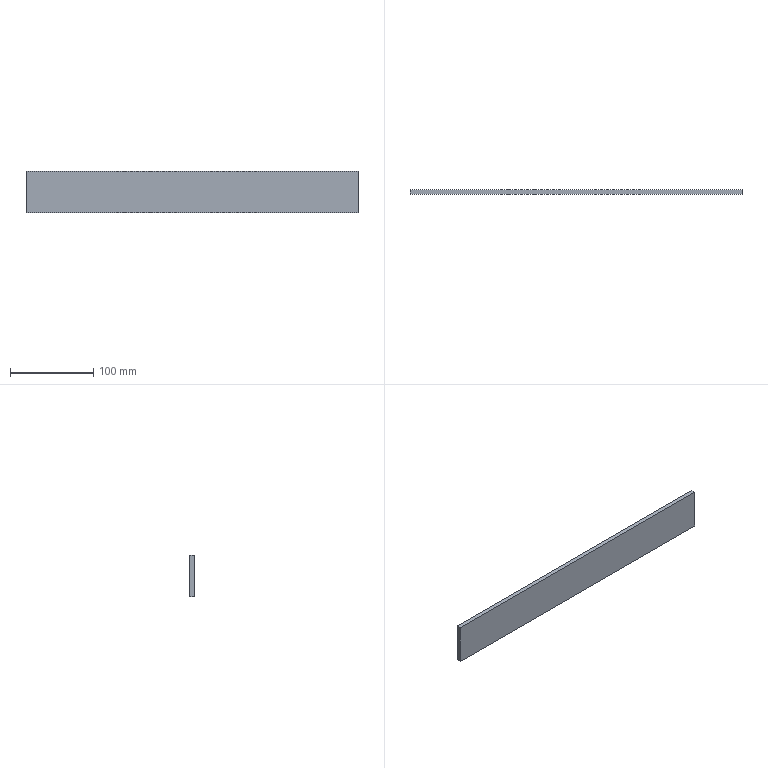Part | SolidWorks | features Extrusion 1 | 1 solid | 6 faces | box 400 x 5 x 50 mm | volume 100000 mm3 | plane 6
STEP:
#1=CARTESIAN_POINT('',(-200.,0.,-25.));
#2=VERTEX_POINT('',#1);
#3=CARTESIAN_POINT('',(-200.,0.,25.));
#4=VERTEX_POINT('',#3);
#5=CARTESIAN_POINT('',(-200.,0.,-25.));
#6=DIRECTION('',(0.,0.,1.));
#7=VECTOR('',#6,1000.);
#8=LINE('',#5,#7);
#9=EDGE_CURVE('',#2,#4,#8,.T.);
#10=ORIENTED_EDGE('',*,*,#9,.T.);
#11=CARTESIAN_POINT('',(-200.,5.,25.));
#12=VERTEX_POINT('',#11);
#13=CARTESIAN_POINT('',(-200.,5.,25.));
#14=DIRECTION('',(0.,-1.,0.));
#15=VECTOR('',#14,1000.);
#16=LINE('',#13,#15);
#17=EDGE_CURVE('',#12,#4,#16,.T.);
#18=ORIENTED_EDGE('',*,*,#17,.F.);
#19=CARTESIAN_POINT('',(-200.,5.,-25.));
#20=VERTEX_POINT('',#19);
#21=CARTESIAN_POINT('',(-200.,5.,-25.));
#22=DIRECTION('',(0.,0.,1.));
#23=VECTOR('',#22,1000.);
#24=LINE('',#21,#23);
#25=EDGE_CURVE('',#20,#12,#24,.T.);
#26=ORIENTED_EDGE('',*,*,#25,.F.);
#27=CARTESIAN_POINT('',(-200.,5.,-25.));
#28=DIRECTION('',(0.,-1.,0.));
#29=VECTOR('',#28,1000.);
#30=LINE('',#27,#29);
#31=EDGE_CURVE('',#20,#2,#30,.T.);
#32=ORIENTED_EDGE('',*,*,#31,.T.);
#33=EDGE_LOOP('',(#10,#18,#26,#32));
#34=FACE_OUTER_BOUND('',#33,.T.);
#35=CARTESIAN_POINT('',(-200.,5.,-25.));
#36=DIRECTION('',(1.,0.,0.));
#37=DIRECTION('',(0.,0.,-1.));
#38=AXIS2_PLACEMENT_3D('',#35,#36,#37);
#39=PLANE('',#38);
#40=ADVANCED_FACE('',(#34),#39,.F.);
#41=CARTESIAN_POINT('',(200.,0.,25.));
#42=VERTEX_POINT('',#41);
#43=CARTESIAN_POINT('',(-200.,0.,25.));
#44=DIRECTION('',(1.,0.,0.));
#45=VECTOR('',#44,1000.);
#46=LINE('',#43,#45);
#47=EDGE_CURVE('',#4,#42,#46,.T.);
#48=ORIENTED_EDGE('',*,*,#47,.T.);
#49=CARTESIAN_POINT('',(200.,5.,25.));
#50=VERTEX_POINT('',#49);
#51=CARTESIAN_POINT('',(200.,5.,25.));
#52=DIRECTION('',(0.,-1.,0.));
#53=VECTOR('',#52,1000.);
#54=LINE('',#51,#53);
#55=EDGE_CURVE('',#50,#42,#54,.T.);
#56=ORIENTED_EDGE('',*,*,#55,.F.);
#57=CARTESIAN_POINT('',(-200.,5.,25.));
#58=DIRECTION('',(1.,0.,0.));
#59=VECTOR('',#58,1000.);
#60=LINE('',#57,#59);
#61=EDGE_CURVE('',#12,#50,#60,.T.);
#62=ORIENTED_EDGE('',*,*,#61,.F.);
#63=ORIENTED_EDGE('',*,*,#17,.T.);
#64=EDGE_LOOP('',(#48,#56,#62,#63));
#65=FACE_OUTER_BOUND('',#64,.T.);
#66=CARTESIAN_POINT('',(-200.,5.,25.));
#67=DIRECTION('',(0.,0.,-1.));
#68=DIRECTION('',(-1.,0.,0.));
#69=AXIS2_PLACEMENT_3D('',#66,#67,#68);
#70=PLANE('',#69);
#71=ADVANCED_FACE('',(#65),#70,.F.);
#72=CARTESIAN_POINT('',(200.,0.,-25.));
#73=VERTEX_POINT('',#72);
#74=CARTESIAN_POINT('',(200.,0.,-25.));
#75=DIRECTION('',(0.,0.,1.));
#76=VECTOR('',#75,1000.);
#77=LINE('',#74,#76);
#78=EDGE_CURVE('',#73,#42,#77,.T.);
#79=ORIENTED_EDGE('',*,*,#78,.F.);
#80=CARTESIAN_POINT('',(200.,5.,-25.));
#81=VERTEX_POINT('',#80);
#82=CARTESIAN_POINT('',(200.,5.,-25.));
#83=DIRECTION('',(0.,-1.,0.));
#84=VECTOR('',#83,1000.);
#85=LINE('',#82,#84);
#86=EDGE_CURVE('',#81,#73,#85,.T.);
#87=ORIENTED_EDGE('',*,*,#86,.F.);
#88=CARTESIAN_POINT('',(200.,5.,-25.));
#89=DIRECTION('',(0.,0.,1.));
#90=VECTOR('',#89,1000.);
#91=LINE('',#88,#90);
#92=EDGE_CURVE('',#81,#50,#91,.T.);
#93=ORIENTED_EDGE('',*,*,#92,.T.);
#94=ORIENTED_EDGE('',*,*,#55,.T.);
#95=EDGE_LOOP('',(#79,#87,#93,#94));
#96=FACE_OUTER_BOUND('',#95,.T.);
#97=CARTESIAN_POINT('',(200.,5.,-25.));
#98=DIRECTION('',(1.,0.,0.));
#99=DIRECTION('',(0.,0.,-1.));
#100=AXIS2_PLACEMENT_3D('',#97,#98,#99);
#101=PLANE('',#100);
#102=ADVANCED_FACE('',(#96),#101,.T.);
#103=CARTESIAN_POINT('',(-200.,0.,-25.));
#104=DIRECTION('',(1.,0.,0.));
#105=VECTOR('',#104,1000.);
#106=LINE('',#103,#105);
#107=EDGE_CURVE('',#2,#73,#106,.T.);
#108=ORIENTED_EDGE('',*,*,#107,.F.);
#109=ORIENTED_EDGE('',*,*,#31,.F.);
#110=CARTESIAN_POINT('',(-200.,5.,-25.));
#111=DIRECTION('',(1.,0.,0.));
#112=VECTOR('',#111,1000.);
#113=LINE('',#110,#112);
#114=EDGE_CURVE('',#20,#81,#113,.T.);
#115=ORIENTED_EDGE('',*,*,#114,.T.);
#116=ORIENTED_EDGE('',*,*,#86,.T.);
#117=EDGE_LOOP('',(#108,#109,#115,#116));
#118=FACE_OUTER_BOUND('',#117,.T.);
#119=CARTESIAN_POINT('',(-200.,5.,-25.));
#120=DIRECTION('',(0.,0.,-1.));
#121=DIRECTION('',(-1.,0.,0.));
#122=AXIS2_PLACEMENT_3D('',#119,#120,#121);
#123=PLANE('',#122);
#124=ADVANCED_FACE('',(#118),#123,.T.);
#125=ORIENTED_EDGE('',*,*,#25,.T.);
#126=ORIENTED_EDGE('',*,*,#61,.T.);
#127=ORIENTED_EDGE('',*,*,#92,.F.);
#128=ORIENTED_EDGE('',*,*,#114,.F.);
#129=EDGE_LOOP('',(#125,#126,#127,#128));
#130=FACE_OUTER_BOUND('',#129,.T.);
#131=CARTESIAN_POINT('',(0.,5.,0.));
#132=DIRECTION('',(0.,1.,0.));
#133=DIRECTION('',(0.,0.,1.));
#134=AXIS2_PLACEMENT_3D('',#131,#132,#133);
#135=PLANE('',#134);
#136=ADVANCED_FACE('',(#130),#135,.T.);
#137=ORIENTED_EDGE('',*,*,#9,.F.);
#138=ORIENTED_EDGE('',*,*,#107,.T.);
#139=ORIENTED_EDGE('',*,*,#78,.T.);
#140=ORIENTED_EDGE('',*,*,#47,.F.);
#141=EDGE_LOOP('',(#137,#138,#139,#140));
#142=FACE_OUTER_BOUND('',#141,.T.);
#143=CARTESIAN_POINT('',(0.,0.,0.));
#144=DIRECTION('',(0.,1.,0.));
#145=DIRECTION('',(0.,0.,1.));
#146=AXIS2_PLACEMENT_3D('',#143,#144,#145);
#147=PLANE('',#146);
#148=ADVANCED_FACE('',(#142),#147,.F.);
#149=CLOSED_SHELL('',(#40,#71,#102,#124,#136,#148));
#150=MANIFOLD_SOLID_BREP('',#149);
#151=CARTESIAN_POINT('',(0.,0.,0.));
#152=DIRECTION('',(0.,0.,1.));
#153=DIRECTION('',(1.,0.,0.));
#154=AXIS2_PLACEMENT_3D('',#151,#152,#153);
#155=(LENGTH_UNIT()NAMED_UNIT(*)SI_UNIT(.MILLI.,.METRE.));
#156=UNCERTAINTY_MEASURE_WITH_UNIT(LENGTH_MEASURE(0.00001),#155,'','');
#157=(NAMED_UNIT(*)PLANE_ANGLE_UNIT()SI_UNIT($,.RADIAN.));
#158=(NAMED_UNIT(*)SI_UNIT($,.STERADIAN.)SOLID_ANGLE_UNIT());
#159=(GEOMETRIC_REPRESENTATION_CONTEXT(3)GLOBAL_UNCERTAINTY_ASSIGNED_CONTEXT((#156))GLOBAL_UNIT_ASSIGNED_CONTEXT((#155,#157,#158))REPRESENTATION_CONTEXT('',''));
#160=ADVANCED_BREP_SHAPE_REPRESENTATION('',(#150,#154),#159);